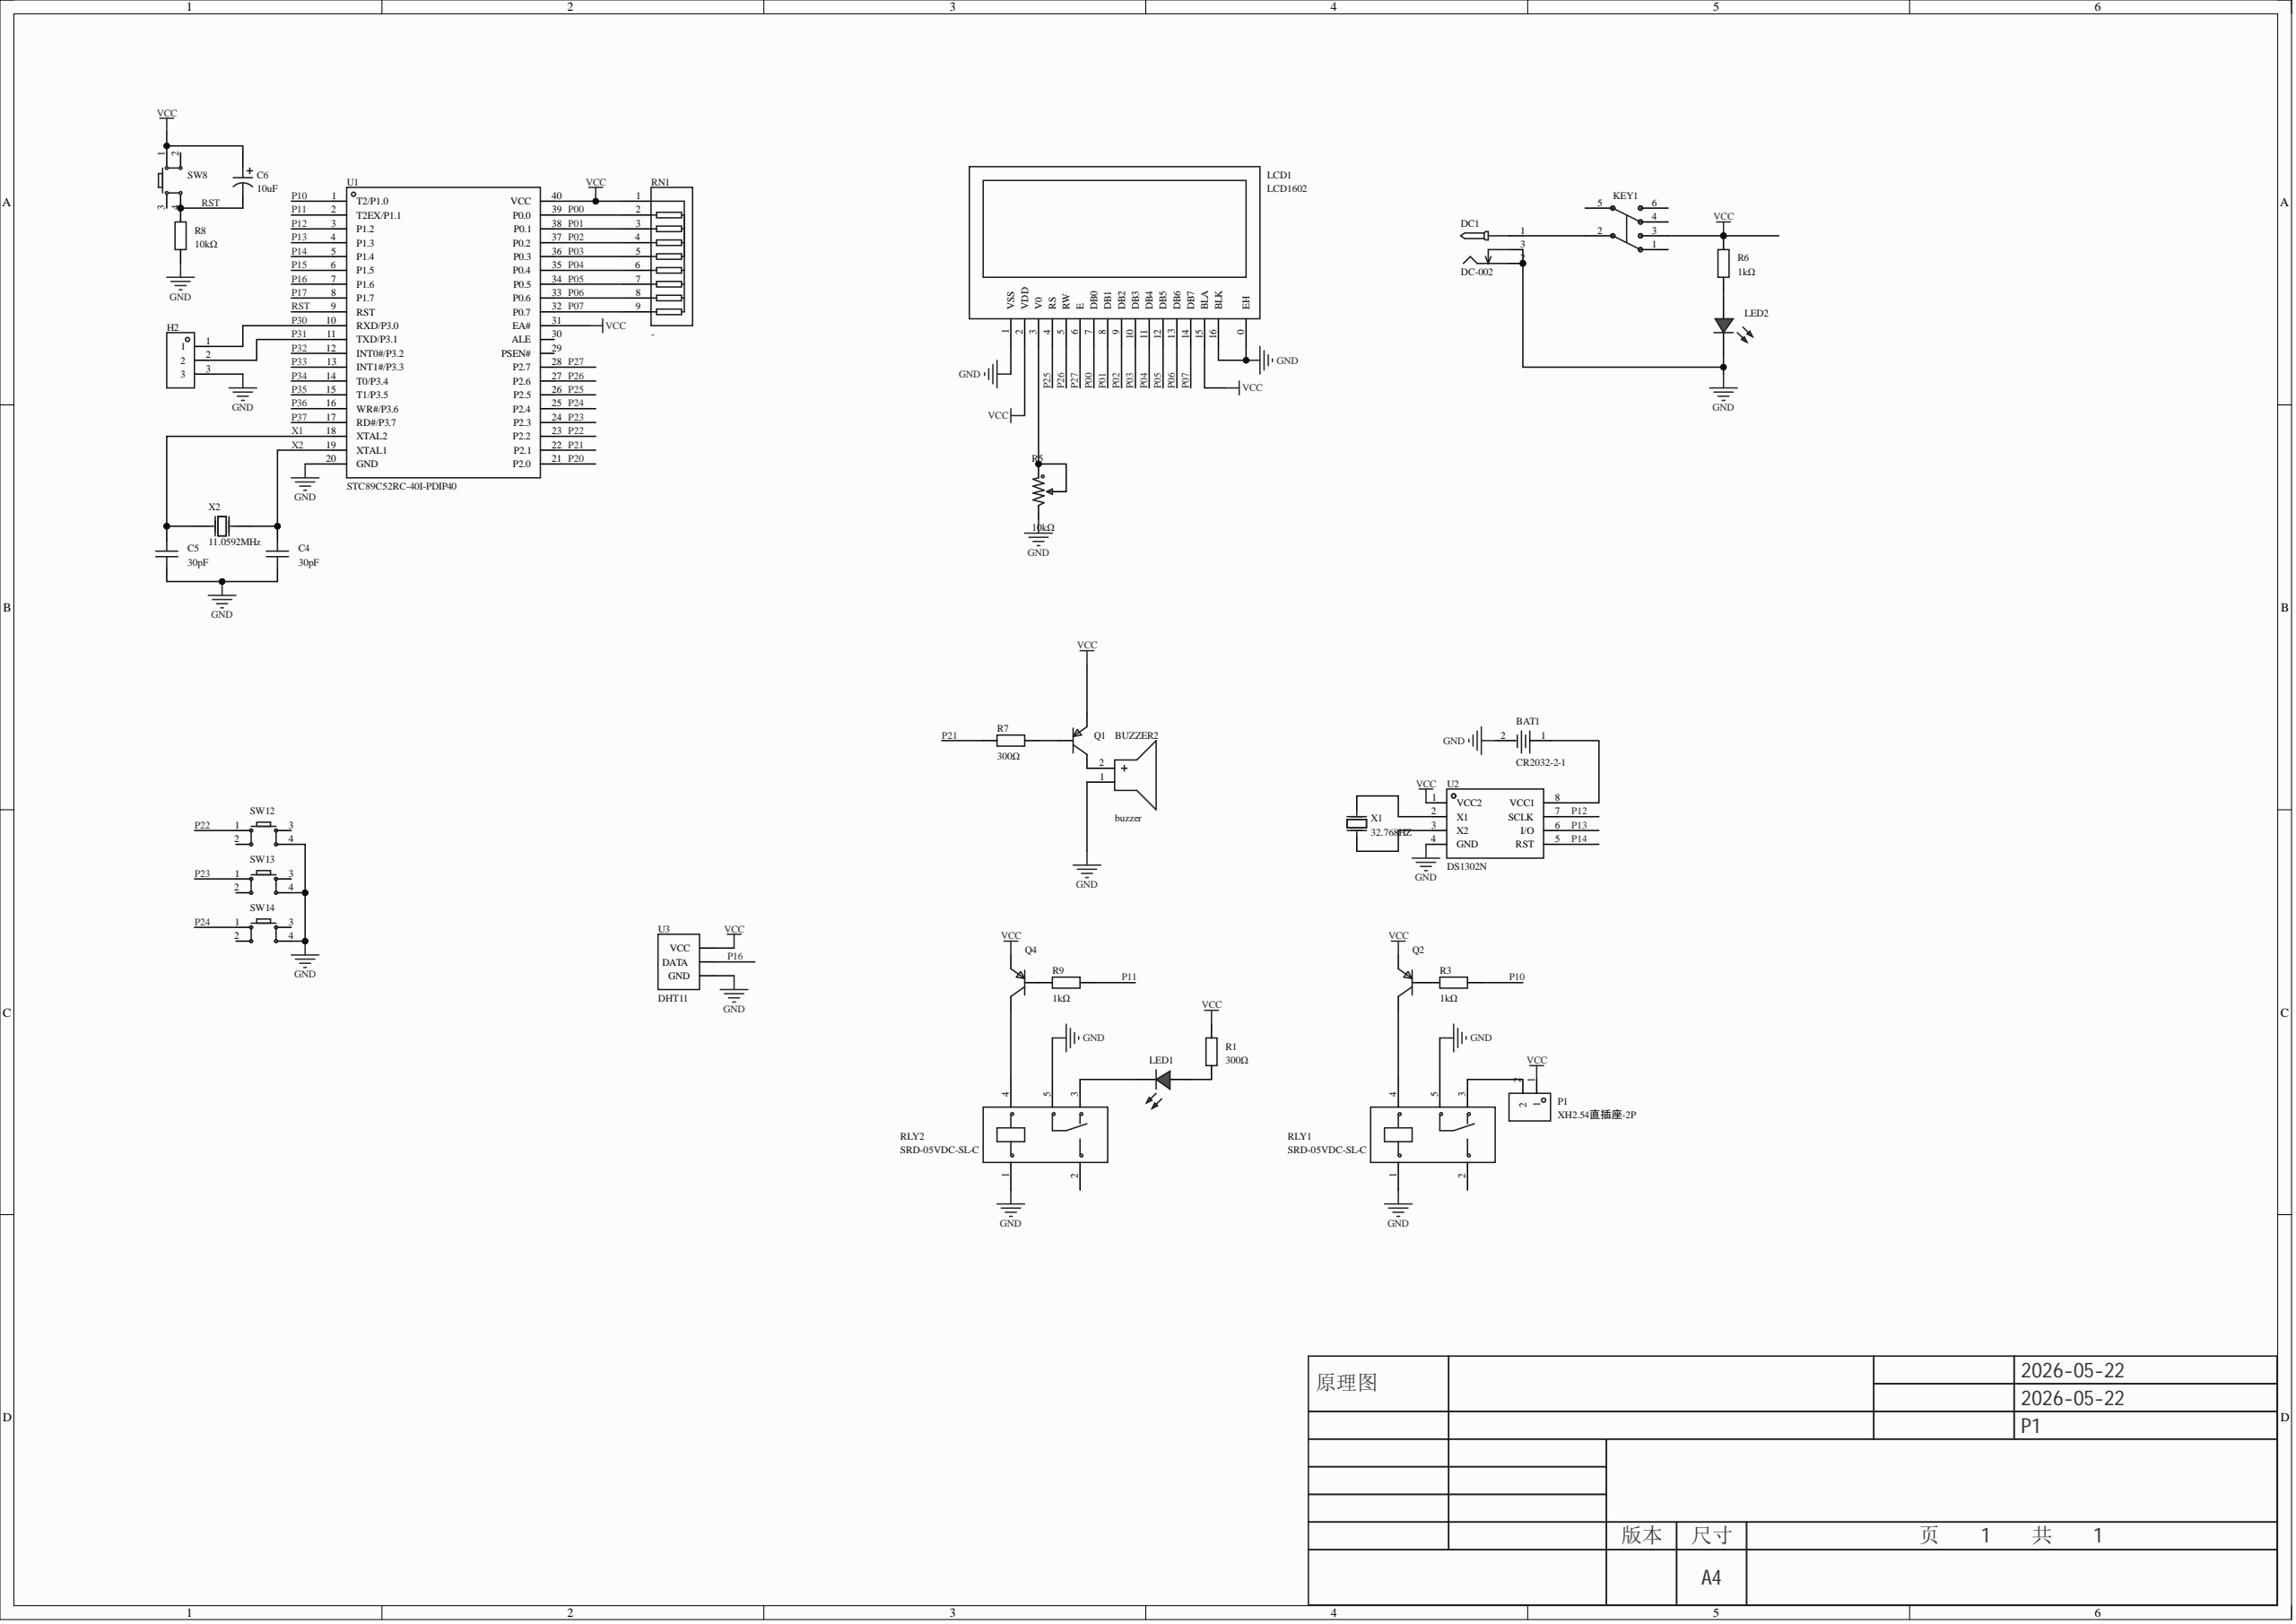Circuit board | Altium Designer | 34 parts | 43 nets
Bill of materials:
Comment,Description,Designator,Footprint,LibRef,Quantity
"CR2032-2-1","","BAT1","BAT-TH_CR2032-2-1","CR2032-2-1","1"
"buzzer","","BUZZER2","BUZ-TH_BD12.0-P6.00-D0.9-RD","buzzer","1"
"30pF","容值:30pF;精度:±10%;额定电压:25V;温度系数:C0G;","C4, C5","CAP-TH_L3.8-W2.5-P2.54-D0.50","C315C300K3G5TA7301","2"
"10uF","","C6","CAP-TH_BD5.0-P2.00-D0.8-FD-10UF50VC110GL","10UF50VC110GL","1"
"DC-002","","DC1","DC-IN-TH_DC-3510","DC-002","1"
"","","H2","HDR-TH_3P-P2.54-V-M","HDR-M_2.54_1x3P","1"
"无自锁开关 8.5×8.5 无声","6脚，8.5×8.5","KEY1","SW-TH_6P-L8.5-W8.5-P2.54","无自锁开关 8.5×8.5 无声","1"
"LCD1602","主控芯片:SPLC780;尺寸(inch):2;","LCD1","LCD1602","HS1602A","1"
"","","LED1, LED2","LED_TH-3mm","LED_TH-R_3mm","2"
"XH2.54直插座-2P","","P1","CONN-TH_XH2.54-2P","XH2.54直插座-2P","1"
"","","Q1, Q2, Q4","S8550P_TO-92","S8550_TO_PNP","3"
"300Ω","","R1, R7","Res_1/8W","Res_AXIAL-1/8W","2"
"1kΩ","","R3, R6, R9","Res_1/8W","Res_AXIAL-1/8W","3"
"10kΩ","","R5","RES-ADJ-SMD_RM065-V1","RM065-103(10K)","1"
"10kΩ","","R8","Res_1/8W","Res_AXIAL-1/8W","1"
"SRD-05VDC-SL-C","线圈电压:5V;触点形式:一组转换:1C(单刀双掷-转换);触点容量(电阻负载):-;最大切换电压:250V@AC;最大切换电流:15A;","RLY1, RLY2","RELAY-TH_SRD-XXVDC-XL-C","SRD-05VDC-SL-C","2"
"-","电阻器数:-;阻值:-;单个元件功率:-;","RN1","RES-ARRAY-TH_9P-P2.54-D1.0","排阻 10 K 5%","1"
"","","SW8, SW12, SW13, SW14","SW-TH_4P-L6.0-W6.0-P4.50-LS6.5","Key_TH_6x6x6","4"
"STC89C52RC-40I-PDIP40","CPU内核:51家族;CPU最大主频:-;","U1","DIP-40_L52.0-W13.7-P2.54-LS15.2-BL","STC89C52RC-40I-PDIP40","1"
"DS1302N","","U2","DIP-8_L9.7-W6.4-P2.54-LS7.6-BL","DS1302N","1"
"DHT11","","U3","DHT11_X","DHT11","1"
"32.768HZ","","X1","HC-49S_L11.5-W5.0-P4.88","8MHZ","1"
"11.059MHz","晶振类型:直插晶振;频率:11.059MHz;常温频差:±20ppm;负载电容:30pF;","X2","OSC-TH_L11.1-W4.7-P4.88","9AC11059302060C3","1"
Netlist (Protel format):
[
BAT1
BAT-TH_CR2032-2-1
CR2032-2-1



]
[
BUZZER2
BUZ-TH_BD12.0-P6.00-D0.9-RD
buzzer



]
[
C4
CAP-TH_L3.8-W2.5-P2.54-D0.50
30pF



]
[
C5
CAP-TH_L3.8-W2.5-P2.54-D0.50
30pF



]
[
C6
CAP-TH_BD5.0-P2.00-D0.8-FD-10UF50VC110GL
10uF



]
[
DC1
DC-IN-TH_DC-3510
DC-002



]
[
H2
HDR-TH_3P-P2.54-V-M




]
[
KEY1
SW-TH_6P-L8.5-W8.5-P2.54
无自锁开关 8.5×8.5 无声



]
[
LCD1
LCD1602
LCD1602



]
[
LED1
LED_TH-3mm




]
[
LED2
LED_TH-3mm




]
[
P1
CONN-TH_XH2.54-2P
XH2.54直插座-2P



]
[
Q1
S8550P_TO-92




]
[
Q2
S8550P_TO-92




]
[
Q4
S8550P_TO-92




]
[
R1
Res_1/8W
300Ω



]
[
R3
Res_1/8W
1kΩ



]
[
R5
RES-ADJ-SMD_RM065-V1
10kΩ



]
[
R6
Res_1/8W
1kΩ



]
[
R7
Res_1/8W
300Ω



]
[
R8
Res_1/8W
10kΩ



]
[
R9
Res_1/8W
1kΩ



]
[
RLY1
RELAY-TH_SRD-XXVDC-XL-C
SRD-05VDC-SL-C



]
[
RLY2
RELAY-TH_SRD-XXVDC-XL-C
SRD-05VDC-SL-C



]
[
RN1
RES-ARRAY-TH_9P-P2.54-D1.0
-



]
[
SW8
SW-TH_4P-L6.0-W6.0-P4.50-LS6.5




]
[
SW12
SW-TH_4P-L6.0-W6.0-P4.50-LS6.5




]
[
SW13
SW-TH_4P-L6.0-W6.0-P4.50-LS6.5




]
[
SW14
SW-TH_4P-L6.0-W6.0-P4.50-LS6.5




]
[
U1
DIP-40_L52.0-W13.7-P2.54-LS15.2-BL
STC89C52RC-40I-PDIP40



]
[
U2
DIP-8_L9.7-W6.4-P2.54-LS7.6-BL
DS1302N



]
[
U3
DHT11_X
DHT11



]
[
X1
HC-49S_L11.5-W5.0-P4.88
32.768HZ



]
[
X2
OSC-TH_L11.1-W4.7-P4.88
11.0592MHz



]
(
X2
C4-2
U1-19
X2-2
)
(
X1
C5-2
U1-18
X2-1
)
(
VCC
C6-1
KEY1-3
LCD1-2
LCD1-15
P1-1
Q1-1
Q2-1
Q4-1
R1-2
R6-2
RN1-1
SW8-1
U1-31
U1-40
U2-1
U3-1
)
(
RST
C6-2
R8-2
SW8-4
U1-9
)
(
P31
H2-2
U1-11
)
(
P30
H2-1
U1-10
)
(
P27
LCD1-6
U1-28
)
(
P26
LCD1-5
U1-27
)
(
P25
LCD1-4
U1-26
)
(
P24
SW14-1
U1-25
)
(
P23
SW13-1
U1-24
)
(
P22
SW12-1
U1-23
)
(
P21
R7-2
U1-22
)
(
P16
U1-7
U3-2
)
(
P14
U1-5
U2-5
)
(
P13
U1-4
U2-6
)
(
P12
U1-3
U2-7
)
(
P11
R9-2
U1-2
)
(
P10
R3-2
U1-1
)
(
P07
LCD1-14
RN1-9
U1-32
)
(
P06
LCD1-13
RN1-8
U1-33
)
(
P05
LCD1-12
RN1-7
U1-34
)
(
P04
LCD1-11
RN1-6
U1-35
)
(
P03
LCD1-10
RN1-5
U1-36
)
(
P02
LCD1-9
RN1-4
U1-37
)
(
P01
LCD1-8
RN1-3
U1-38
)
(
P00
LCD1-7
RN1-2
U1-39
)
(
NetU2_3
U2-3
X1-1
)
(
NetU2_2
U2-2
X1-2
)
(
NetQ4_3
Q4-3
RLY2-4
)
(
NetQ4_2
Q4-2
R9-1
)
(
NetQ2_3
Q2-3
RLY1-4
)
(
NetQ2_2
Q2-2
R3-1
)
(
NetQ1_2
Q1-2
R7-1
)
(
NetP1_2
P1-2
RLY1-3
)
(
NetLED2_1
LED2-1
R6-1
)
(
NetLED1_2
LED1-2
RLY2-3
)
(
NetLED1_1
LED1-1
R1-1
)
(
NetLCD1_3
LCD1-3
R5-1
R5-2
)
(
NetDC1_1
DC1-1
KEY1-2
)
(
NetBUZZER2_2
BUZZER2-2
Q1-3
)
(
NetBAT1_1
BAT1-1
U2-8
)
(
GND
BAT1-2
BUZZER2-1
C4-1
C5-1
DC1-2
DC1-3
H2-3
LCD1-0
LCD1-1
LCD1-16
LED2-2
R5-3
R8-1
RLY1-1
RLY1-5
RLY2-1
RLY2-5
SW12-4
SW13-4
SW14-4
U1-20
U2-4
U3-3
)